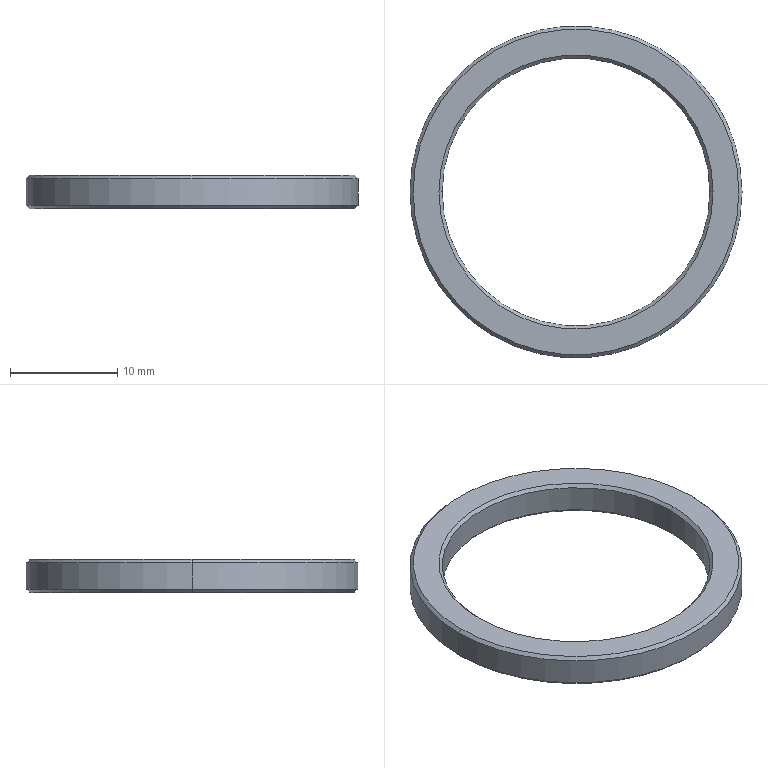Part | NX | 1 solid | 14 faces | box 31 x 31 x 3.1 mm | volume 802.237 mm3 | cone 8 | cylinder 4 | plane 2 | commonest cylinder face diameters 25 x2 31 x2
STEP:
#1=CARTESIAN_POINT('',(-307.373,1008.5,-190.983));
#2=VERTEX_POINT('',#1);
#3=CARTESIAN_POINT('',(-282.373,1008.5,-190.983));
#4=VERTEX_POINT('',#3);
#5=CARTESIAN_POINT('',(-294.873,1008.5,-190.983));
#6=DIRECTION('',(0.,0.,1.));
#7=DIRECTION('',(1.,0.,0.));
#8=AXIS2_PLACEMENT_3D('',#5,#6,#7);
#9=CIRCLE('',#8,12.5);
#10=EDGE_CURVE('',#2,#4,#9,.T.);
#11=ORIENTED_EDGE('',*,*,#10,.T.);
#12=CARTESIAN_POINT('',(-282.373,1008.5,-193.483));
#13=VERTEX_POINT('',#12);
#14=CARTESIAN_POINT('',(-282.373,1008.5,-194.783));
#15=DIRECTION('',(0.,0.,-1.));
#16=VECTOR('',#15,1000.);
#17=LINE('',#14,#16);
#18=EDGE_CURVE('',#4,#13,#17,.T.);
#19=ORIENTED_EDGE('',*,*,#18,.T.);
#20=CARTESIAN_POINT('',(-307.373,1008.5,-193.483));
#21=VERTEX_POINT('',#20);
#22=CARTESIAN_POINT('',(-294.873,1008.5,-193.483));
#23=DIRECTION('',(0.,0.,-1.));
#24=DIRECTION('',(-1.,0.,0.));
#25=AXIS2_PLACEMENT_3D('',#22,#23,#24);
#26=CIRCLE('',#25,12.5);
#27=EDGE_CURVE('',#13,#21,#26,.T.);
#28=ORIENTED_EDGE('',*,*,#27,.T.);
#29=CARTESIAN_POINT('',(-307.373,1008.5,-194.783));
#30=DIRECTION('',(0.,0.,-1.));
#31=VECTOR('',#30,1000.);
#32=LINE('',#29,#31);
#33=EDGE_CURVE('',#2,#21,#32,.T.);
#34=ORIENTED_EDGE('',*,*,#33,.F.);
#35=EDGE_LOOP('',(#11,#19,#28,#34));
#36=FACE_BOUND('',#35,.T.);
#37=CARTESIAN_POINT('',(-294.873,1008.5,-194.783));
#38=DIRECTION('',(0.,0.,-1.));
#39=DIRECTION('',(1.,0.,0.));
#40=AXIS2_PLACEMENT_3D('',#37,#38,#39);
#41=CYLINDRICAL_SURFACE('',#40,12.5);
#42=ADVANCED_FACE('',(#36),#41,.F.);
#43=CARTESIAN_POINT('',(-294.873,1008.5,-193.483));
#44=DIRECTION('',(0.,0.,-1.));
#45=DIRECTION('',(-1.,0.,0.));
#46=AXIS2_PLACEMENT_3D('',#43,#44,#45);
#47=CIRCLE('',#46,12.5);
#48=EDGE_CURVE('',#21,#13,#47,.T.);
#49=ORIENTED_EDGE('',*,*,#48,.F.);
#50=CARTESIAN_POINT('',(-307.673,1008.5,-193.783));
#51=VERTEX_POINT('',#50);
#52=CARTESIAN_POINT('',(-307.673,1008.5,-193.783));
#53=DIRECTION('',(-0.7071,0.,-0.7071));
#54=VECTOR('',#53,1000.);
#55=LINE('',#52,#54);
#56=EDGE_CURVE('',#51,#21,#55,.F.);
#57=ORIENTED_EDGE('',*,*,#56,.F.);
#58=CARTESIAN_POINT('',(-282.073,1008.5,-193.783));
#59=VERTEX_POINT('',#58);
#60=CARTESIAN_POINT('',(-294.873,1008.5,-193.783));
#61=DIRECTION('',(0.,0.,-1.));
#62=DIRECTION('',(-1.,0.,0.));
#63=AXIS2_PLACEMENT_3D('',#60,#61,#62);
#64=CIRCLE('',#63,12.8);
#65=EDGE_CURVE('',#51,#59,#64,.T.);
#66=ORIENTED_EDGE('',*,*,#65,.T.);
#67=CARTESIAN_POINT('',(-282.073,1008.5,-193.783));
#68=DIRECTION('',(0.7071,0.,-0.7071));
#69=VECTOR('',#68,1000.);
#70=LINE('',#67,#69);
#71=EDGE_CURVE('',#59,#13,#70,.F.);
#72=ORIENTED_EDGE('',*,*,#71,.T.);
#73=EDGE_LOOP('',(#49,#57,#66,#72));
#74=FACE_BOUND('',#73,.T.);
#75=CARTESIAN_POINT('',(-294.873,1008.5,-193.783));
#76=DIRECTION('',(0.,0.,-1.));
#77=DIRECTION('',(-1.,0.,0.));
#78=AXIS2_PLACEMENT_3D('',#75,#76,#77);
#79=CONICAL_SURFACE('',#78,12.8,0.7854);
#80=ADVANCED_FACE('',(#74),#79,.F.);
#81=CARTESIAN_POINT('',(-279.373,1008.5,-190.983));
#82=VERTEX_POINT('',#81);
#83=CARTESIAN_POINT('',(-310.373,1008.5,-190.983));
#84=VERTEX_POINT('',#83);
#85=CARTESIAN_POINT('',(-294.873,1008.5,-190.983));
#86=DIRECTION('',(0.,0.,-1.));
#87=DIRECTION('',(-1.,0.,0.));
#88=AXIS2_PLACEMENT_3D('',#85,#86,#87);
#89=CIRCLE('',#88,15.5);
#90=EDGE_CURVE('',#82,#84,#89,.T.);
#91=ORIENTED_EDGE('',*,*,#90,.T.);
#92=CARTESIAN_POINT('',(-310.373,1008.5,-193.483));
#93=VERTEX_POINT('',#92);
#94=CARTESIAN_POINT('',(-310.373,1008.5,-194.783));
#95=DIRECTION('',(0.,0.,-1.));
#96=VECTOR('',#95,1000.);
#97=LINE('',#94,#96);
#98=EDGE_CURVE('',#93,#84,#97,.F.);
#99=ORIENTED_EDGE('',*,*,#98,.F.);
#100=CARTESIAN_POINT('',(-279.373,1008.5,-193.483));
#101=VERTEX_POINT('',#100);
#102=CARTESIAN_POINT('',(-294.873,1008.5,-193.483));
#103=DIRECTION('',(0.,0.,1.));
#104=DIRECTION('',(1.,0.,0.));
#105=AXIS2_PLACEMENT_3D('',#102,#103,#104);
#106=CIRCLE('',#105,15.5);
#107=EDGE_CURVE('',#93,#101,#106,.T.);
#108=ORIENTED_EDGE('',*,*,#107,.T.);
#109=CARTESIAN_POINT('',(-279.373,1008.5,-194.783));
#110=DIRECTION('',(0.,0.,-1.));
#111=VECTOR('',#110,1000.);
#112=LINE('',#109,#111);
#113=EDGE_CURVE('',#101,#82,#112,.F.);
#114=ORIENTED_EDGE('',*,*,#113,.T.);
#115=EDGE_LOOP('',(#91,#99,#108,#114));
#116=FACE_BOUND('',#115,.T.);
#117=CARTESIAN_POINT('',(-294.873,1008.5,-194.783));
#118=DIRECTION('',(0.,0.,-1.));
#119=DIRECTION('',(-1.,0.,0.));
#120=AXIS2_PLACEMENT_3D('',#117,#118,#119);
#121=CYLINDRICAL_SURFACE('',#120,15.5);
#122=ADVANCED_FACE('',(#116),#121,.T.);
#123=CARTESIAN_POINT('',(-310.073,1008.5,-193.783));
#124=VERTEX_POINT('',#123);
#125=CARTESIAN_POINT('',(-279.673,1008.5,-193.783));
#126=VERTEX_POINT('',#125);
#127=CARTESIAN_POINT('',(-294.873,1008.5,-193.783));
#128=DIRECTION('',(0.,0.,1.));
#129=DIRECTION('',(1.,0.,0.));
#130=AXIS2_PLACEMENT_3D('',#127,#128,#129);
#131=CIRCLE('',#130,15.2);
#132=EDGE_CURVE('',#124,#126,#131,.T.);
#133=ORIENTED_EDGE('',*,*,#132,.F.);
#134=CARTESIAN_POINT('',(-294.873,1008.5,-193.783));
#135=DIRECTION('',(0.,0.,1.));
#136=DIRECTION('',(1.,0.,0.));
#137=AXIS2_PLACEMENT_3D('',#134,#135,#136);
#138=CIRCLE('',#137,15.2);
#139=EDGE_CURVE('',#126,#124,#138,.T.);
#140=ORIENTED_EDGE('',*,*,#139,.F.);
#141=EDGE_LOOP('',(#133,#140));
#142=FACE_BOUND('',#141,.T.);
#143=CARTESIAN_POINT('',(-294.873,1008.5,-193.783));
#144=DIRECTION('',(0.,0.,-1.));
#145=DIRECTION('',(-1.,0.,0.));
#146=AXIS2_PLACEMENT_3D('',#143,#144,#145);
#147=CIRCLE('',#146,12.8);
#148=EDGE_CURVE('',#59,#51,#147,.T.);
#149=ORIENTED_EDGE('',*,*,#148,.F.);
#150=ORIENTED_EDGE('',*,*,#65,.F.);
#151=EDGE_LOOP('',(#149,#150));
#152=FACE_BOUND('',#151,.T.);
#153=CARTESIAN_POINT('',(-291.163,1020.145,-193.783));
#154=DIRECTION('',(0.,0.,-1.));
#155=DIRECTION('',(0.,-1.,0.));
#156=AXIS2_PLACEMENT_3D('',#153,#154,#155);
#157=PLANE('',#156);
#158=ADVANCED_FACE('',(#142,#152),#157,.T.);
#159=CARTESIAN_POINT('',(-279.673,1008.5,-190.683));
#160=VERTEX_POINT('',#159);
#161=CARTESIAN_POINT('',(-310.073,1008.5,-190.683));
#162=VERTEX_POINT('',#161);
#163=CARTESIAN_POINT('',(-294.873,1008.5,-190.683));
#164=DIRECTION('',(0.,0.,-1.));
#165=DIRECTION('',(-1.,0.,0.));
#166=AXIS2_PLACEMENT_3D('',#163,#164,#165);
#167=CIRCLE('',#166,15.2);
#168=EDGE_CURVE('',#160,#162,#167,.T.);
#169=ORIENTED_EDGE('',*,*,#168,.F.);
#170=CARTESIAN_POINT('',(-294.873,1008.5,-190.683));
#171=DIRECTION('',(0.,0.,-1.));
#172=DIRECTION('',(-1.,0.,0.));
#173=AXIS2_PLACEMENT_3D('',#170,#171,#172);
#174=CIRCLE('',#173,15.2);
#175=EDGE_CURVE('',#162,#160,#174,.T.);
#176=ORIENTED_EDGE('',*,*,#175,.F.);
#177=EDGE_LOOP('',(#169,#176));
#178=FACE_BOUND('',#177,.T.);
#179=CARTESIAN_POINT('',(-282.073,1008.5,-190.683));
#180=VERTEX_POINT('',#179);
#181=CARTESIAN_POINT('',(-307.673,1008.5,-190.683));
#182=VERTEX_POINT('',#181);
#183=CARTESIAN_POINT('',(-294.873,1008.5,-190.683));
#184=DIRECTION('',(0.,0.,1.));
#185=DIRECTION('',(1.,0.,0.));
#186=AXIS2_PLACEMENT_3D('',#183,#184,#185);
#187=CIRCLE('',#186,12.8);
#188=EDGE_CURVE('',#180,#182,#187,.T.);
#189=ORIENTED_EDGE('',*,*,#188,.F.);
#190=CARTESIAN_POINT('',(-294.873,1008.5,-190.683));
#191=DIRECTION('',(0.,0.,1.));
#192=DIRECTION('',(1.,0.,0.));
#193=AXIS2_PLACEMENT_3D('',#190,#191,#192);
#194=CIRCLE('',#193,12.8);
#195=EDGE_CURVE('',#182,#180,#194,.T.);
#196=ORIENTED_EDGE('',*,*,#195,.F.);
#197=EDGE_LOOP('',(#189,#196));
#198=FACE_BOUND('',#197,.T.);
#199=CARTESIAN_POINT('',(-291.163,1020.145,-190.683));
#200=DIRECTION('',(0.,0.,-1.));
#201=DIRECTION('',(0.,-1.,0.));
#202=AXIS2_PLACEMENT_3D('',#199,#200,#201);
#203=PLANE('',#202);
#204=ADVANCED_FACE('',(#178,#198),#203,.F.);
#205=ORIENTED_EDGE('',*,*,#188,.T.);
#206=CARTESIAN_POINT('',(-307.673,1008.5,-190.683));
#207=DIRECTION('',(-0.7071,0.,0.7071));
#208=VECTOR('',#207,1000.);
#209=LINE('',#206,#208);
#210=EDGE_CURVE('',#182,#2,#209,.F.);
#211=ORIENTED_EDGE('',*,*,#210,.T.);
#212=CARTESIAN_POINT('',(-294.873,1008.5,-190.983));
#213=DIRECTION('',(0.,0.,1.));
#214=DIRECTION('',(1.,0.,0.));
#215=AXIS2_PLACEMENT_3D('',#212,#213,#214);
#216=CIRCLE('',#215,12.5);
#217=EDGE_CURVE('',#4,#2,#216,.T.);
#218=ORIENTED_EDGE('',*,*,#217,.F.);
#219=CARTESIAN_POINT('',(-282.073,1008.5,-190.683));
#220=DIRECTION('',(0.7071,0.,0.7071));
#221=VECTOR('',#220,1000.);
#222=LINE('',#219,#221);
#223=EDGE_CURVE('',#180,#4,#222,.F.);
#224=ORIENTED_EDGE('',*,*,#223,.F.);
#225=EDGE_LOOP('',(#205,#211,#218,#224));
#226=FACE_BOUND('',#225,.T.);
#227=CARTESIAN_POINT('',(-294.873,1008.5,-190.683));
#228=DIRECTION('',(0.,0.,1.));
#229=DIRECTION('',(1.,0.,0.));
#230=AXIS2_PLACEMENT_3D('',#227,#228,#229);
#231=CONICAL_SURFACE('',#230,12.8,0.7854);
#232=ADVANCED_FACE('',(#226),#231,.F.);
#233=ORIENTED_EDGE('',*,*,#90,.F.);
#234=CARTESIAN_POINT('',(-279.673,1008.5,-190.683));
#235=DIRECTION('',(0.7071,0.,-0.7071));
#236=VECTOR('',#235,1000.);
#237=LINE('',#234,#236);
#238=EDGE_CURVE('',#82,#160,#237,.F.);
#239=ORIENTED_EDGE('',*,*,#238,.T.);
#240=ORIENTED_EDGE('',*,*,#168,.T.);
#241=CARTESIAN_POINT('',(-310.073,1008.5,-190.683));
#242=DIRECTION('',(-0.7071,0.,-0.7071));
#243=VECTOR('',#242,1000.);
#244=LINE('',#241,#243);
#245=EDGE_CURVE('',#84,#162,#244,.F.);
#246=ORIENTED_EDGE('',*,*,#245,.F.);
#247=EDGE_LOOP('',(#233,#239,#240,#246));
#248=FACE_BOUND('',#247,.T.);
#249=CARTESIAN_POINT('',(-294.873,1008.5,-190.683));
#250=DIRECTION('',(0.,0.,-1.));
#251=DIRECTION('',(-1.,0.,0.));
#252=AXIS2_PLACEMENT_3D('',#249,#250,#251);
#253=CONICAL_SURFACE('',#252,15.2,0.7854);
#254=ADVANCED_FACE('',(#248),#253,.T.);
#255=ORIENTED_EDGE('',*,*,#132,.T.);
#256=CARTESIAN_POINT('',(-279.673,1008.5,-193.783));
#257=DIRECTION('',(0.7071,0.,0.7071));
#258=VECTOR('',#257,1000.);
#259=LINE('',#256,#258);
#260=EDGE_CURVE('',#126,#101,#259,.T.);
#261=ORIENTED_EDGE('',*,*,#260,.T.);
#262=ORIENTED_EDGE('',*,*,#107,.F.);
#263=CARTESIAN_POINT('',(-310.073,1008.5,-193.783));
#264=DIRECTION('',(-0.7071,0.,0.7071));
#265=VECTOR('',#264,1000.);
#266=LINE('',#263,#265);
#267=EDGE_CURVE('',#124,#93,#266,.T.);
#268=ORIENTED_EDGE('',*,*,#267,.F.);
#269=EDGE_LOOP('',(#255,#261,#262,#268));
#270=FACE_BOUND('',#269,.T.);
#271=CARTESIAN_POINT('',(-294.873,1008.5,-193.783));
#272=DIRECTION('',(0.,0.,1.));
#273=DIRECTION('',(1.,0.,0.));
#274=AXIS2_PLACEMENT_3D('',#271,#272,#273);
#275=CONICAL_SURFACE('',#274,15.2,0.7854);
#276=ADVANCED_FACE('',(#270),#275,.T.);
#277=ORIENTED_EDGE('',*,*,#245,.T.);
#278=ORIENTED_EDGE('',*,*,#175,.T.);
#279=ORIENTED_EDGE('',*,*,#238,.F.);
#280=CARTESIAN_POINT('',(-294.873,1008.5,-190.983));
#281=DIRECTION('',(0.,0.,-1.));
#282=DIRECTION('',(-1.,0.,0.));
#283=AXIS2_PLACEMENT_3D('',#280,#281,#282);
#284=CIRCLE('',#283,15.5);
#285=EDGE_CURVE('',#84,#82,#284,.T.);
#286=ORIENTED_EDGE('',*,*,#285,.F.);
#287=EDGE_LOOP('',(#277,#278,#279,#286));
#288=FACE_BOUND('',#287,.T.);
#289=CARTESIAN_POINT('',(-294.873,1008.5,-190.683));
#290=DIRECTION('',(0.,0.,-1.));
#291=DIRECTION('',(-1.,0.,0.));
#292=AXIS2_PLACEMENT_3D('',#289,#290,#291);
#293=CONICAL_SURFACE('',#292,15.2,0.7854);
#294=ADVANCED_FACE('',(#288),#293,.T.);
#295=ORIENTED_EDGE('',*,*,#48,.T.);
#296=ORIENTED_EDGE('',*,*,#18,.F.);
#297=ORIENTED_EDGE('',*,*,#217,.T.);
#298=ORIENTED_EDGE('',*,*,#33,.T.);
#299=EDGE_LOOP('',(#295,#296,#297,#298));
#300=FACE_BOUND('',#299,.T.);
#301=CARTESIAN_POINT('',(-294.873,1008.5,-194.783));
#302=DIRECTION('',(0.,0.,-1.));
#303=DIRECTION('',(1.,0.,0.));
#304=AXIS2_PLACEMENT_3D('',#301,#302,#303);
#305=CYLINDRICAL_SURFACE('',#304,12.5);
#306=ADVANCED_FACE('',(#300),#305,.F.);
#307=ORIENTED_EDGE('',*,*,#148,.T.);
#308=ORIENTED_EDGE('',*,*,#56,.T.);
#309=ORIENTED_EDGE('',*,*,#27,.F.);
#310=ORIENTED_EDGE('',*,*,#71,.F.);
#311=EDGE_LOOP('',(#307,#308,#309,#310));
#312=FACE_BOUND('',#311,.T.);
#313=CARTESIAN_POINT('',(-294.873,1008.5,-193.783));
#314=DIRECTION('',(0.,0.,-1.));
#315=DIRECTION('',(-1.,0.,0.));
#316=AXIS2_PLACEMENT_3D('',#313,#314,#315);
#317=CONICAL_SURFACE('',#316,12.8,0.7854);
#318=ADVANCED_FACE('',(#312),#317,.F.);
#319=ORIENTED_EDGE('',*,*,#98,.T.);
#320=ORIENTED_EDGE('',*,*,#285,.T.);
#321=ORIENTED_EDGE('',*,*,#113,.F.);
#322=CARTESIAN_POINT('',(-294.873,1008.5,-193.483));
#323=DIRECTION('',(0.,0.,1.));
#324=DIRECTION('',(1.,0.,0.));
#325=AXIS2_PLACEMENT_3D('',#322,#323,#324);
#326=CIRCLE('',#325,15.5);
#327=EDGE_CURVE('',#101,#93,#326,.T.);
#328=ORIENTED_EDGE('',*,*,#327,.T.);
#329=EDGE_LOOP('',(#319,#320,#321,#328));
#330=FACE_BOUND('',#329,.T.);
#331=CARTESIAN_POINT('',(-294.873,1008.5,-194.783));
#332=DIRECTION('',(0.,0.,-1.));
#333=DIRECTION('',(-1.,0.,0.));
#334=AXIS2_PLACEMENT_3D('',#331,#332,#333);
#335=CYLINDRICAL_SURFACE('',#334,15.5);
#336=ADVANCED_FACE('',(#330),#335,.T.);
#337=ORIENTED_EDGE('',*,*,#10,.F.);
#338=ORIENTED_EDGE('',*,*,#210,.F.);
#339=ORIENTED_EDGE('',*,*,#195,.T.);
#340=ORIENTED_EDGE('',*,*,#223,.T.);
#341=EDGE_LOOP('',(#337,#338,#339,#340));
#342=FACE_BOUND('',#341,.T.);
#343=CARTESIAN_POINT('',(-294.873,1008.5,-190.683));
#344=DIRECTION('',(0.,0.,1.));
#345=DIRECTION('',(1.,0.,0.));
#346=AXIS2_PLACEMENT_3D('',#343,#344,#345);
#347=CONICAL_SURFACE('',#346,12.8,0.7854);
#348=ADVANCED_FACE('',(#342),#347,.F.);
#349=ORIENTED_EDGE('',*,*,#260,.F.);
#350=ORIENTED_EDGE('',*,*,#139,.T.);
#351=ORIENTED_EDGE('',*,*,#267,.T.);
#352=ORIENTED_EDGE('',*,*,#327,.F.);
#353=EDGE_LOOP('',(#349,#350,#351,#352));
#354=FACE_BOUND('',#353,.T.);
#355=CARTESIAN_POINT('',(-294.873,1008.5,-193.783));
#356=DIRECTION('',(0.,0.,1.));
#357=DIRECTION('',(1.,0.,0.));
#358=AXIS2_PLACEMENT_3D('',#355,#356,#357);
#359=CONICAL_SURFACE('',#358,15.2,0.7854);
#360=ADVANCED_FACE('',(#354),#359,.T.);
#361=CLOSED_SHELL('',(#42,#80,#122,#158,#204,#232,#254,#276,#294,#306,#318,#336,#348,#360));
#362=MANIFOLD_SOLID_BREP('',#361);
#363=(LENGTH_UNIT()NAMED_UNIT(*)SI_UNIT(.MILLI.,.METRE.));
#364=UNCERTAINTY_MEASURE_WITH_UNIT(LENGTH_MEASURE(0.00001),#363,'','');
#365=(NAMED_UNIT(*)PLANE_ANGLE_UNIT()SI_UNIT($,.RADIAN.));
#366=(NAMED_UNIT(*)SI_UNIT($,.STERADIAN.)SOLID_ANGLE_UNIT());
#367=(GEOMETRIC_REPRESENTATION_CONTEXT(3)GLOBAL_UNCERTAINTY_ASSIGNED_CONTEXT((#364))GLOBAL_UNIT_ASSIGNED_CONTEXT((#363,#365,#366))REPRESENTATION_CONTEXT('',''));
#368=ADVANCED_BREP_SHAPE_REPRESENTATION('',(#362),#367);